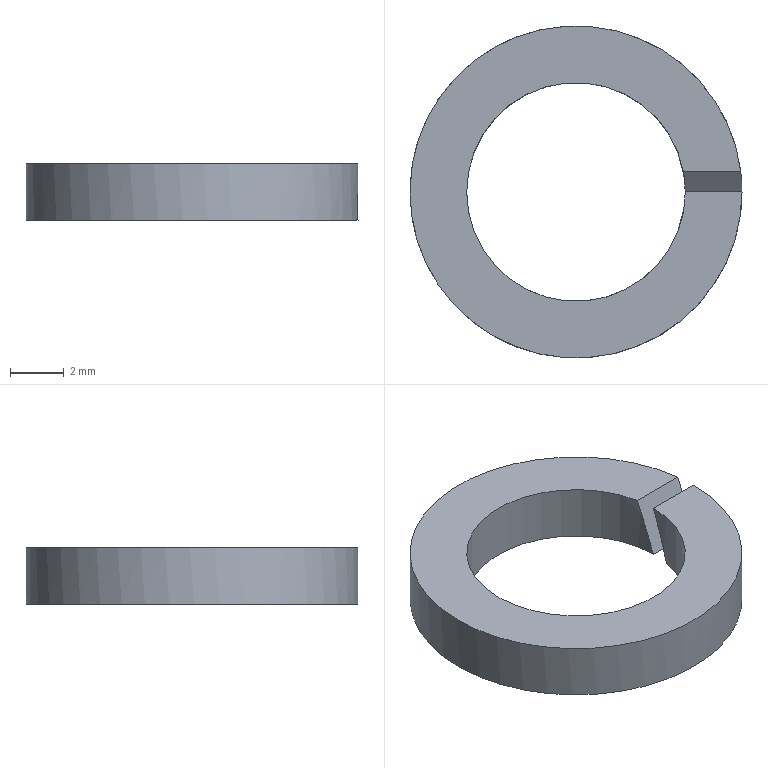Part | NX | features DATUM_CSYS 3, EXTRUDE 2, SKETCH 2 | 1 solid | 6 faces | box 12.3 x 12.3 x 2.1 mm | volume 137.929 mm3 | plane 4 | cylinder 2 | commonest cylinder face diameters 8.1 x1 12.3 x1
STEP:
#1=CARTESIAN_POINT('',(6.15,0.0009353,-1.05));
#2=VERTEX_POINT('',#1);
#3=CARTESIAN_POINT('',(6.102,0.7653,1.05));
#4=VERTEX_POINT('',#3);
#5=CARTESIAN_POINT('',(0.,0.,-1.053));
#6=DIRECTION('',(0.,-0.9397,0.342));
#7=DIRECTION('',(0.,-0.342,-0.9397));
#8=AXIS2_PLACEMENT_3D('',#5,#6,#7);
#9=ELLIPSE('',#8,17.981,6.15);
#10=EDGE_CURVE('',#2,#4,#9,.T.);
#11=ORIENTED_EDGE('',*,*,#10,.F.);
#12=CARTESIAN_POINT('',(6.102,-0.7653,-1.05));
#13=VERTEX_POINT('',#12);
#14=CARTESIAN_POINT('',(0.,0.,-1.05));
#15=DIRECTION('',(0.,0.,1.));
#16=DIRECTION('',(1.,0.,0.));
#17=AXIS2_PLACEMENT_3D('',#14,#15,#16);
#18=CIRCLE('',#17,6.15);
#19=EDGE_CURVE('',#2,#13,#18,.T.);
#20=ORIENTED_EDGE('',*,*,#19,.T.);
#21=CARTESIAN_POINT('',(6.15,-0.0009353,1.05));
#22=VERTEX_POINT('',#21);
#23=CARTESIAN_POINT('',(0.,0.,1.053));
#24=DIRECTION('',(0.,0.9397,-0.342));
#25=DIRECTION('',(0.,-0.342,-0.9397));
#26=AXIS2_PLACEMENT_3D('',#23,#24,#25);
#27=ELLIPSE('',#26,17.981,6.15);
#28=EDGE_CURVE('',#22,#13,#27,.T.);
#29=ORIENTED_EDGE('',*,*,#28,.F.);
#30=CARTESIAN_POINT('',(0.,0.,1.05));
#31=DIRECTION('',(0.,0.,1.));
#32=DIRECTION('',(1.,0.,0.));
#33=AXIS2_PLACEMENT_3D('',#30,#31,#32);
#34=CIRCLE('',#33,6.15);
#35=EDGE_CURVE('',#4,#22,#34,.T.);
#36=ORIENTED_EDGE('',*,*,#35,.F.);
#37=EDGE_LOOP('',(#11,#20,#29,#36));
#38=FACE_BOUND('',#37,.T.);
#39=CARTESIAN_POINT('',(0.,0.,1.05));
#40=DIRECTION('',(0.,0.,-1.));
#41=DIRECTION('',(-1.,0.,0.));
#42=AXIS2_PLACEMENT_3D('',#39,#40,#41);
#43=CYLINDRICAL_SURFACE('',#42,6.15);
#44=ADVANCED_FACE('',(#38),#43,.T.);
#45=CARTESIAN_POINT('',(4.05,0.0009353,-1.05));
#46=VERTEX_POINT('',#45);
#47=CARTESIAN_POINT('',(3.977,-0.7653,-1.05));
#48=VERTEX_POINT('',#47);
#49=CARTESIAN_POINT('',(0.,0.,-1.05));
#50=DIRECTION('',(0.,0.,1.));
#51=DIRECTION('',(1.,0.,0.));
#52=AXIS2_PLACEMENT_3D('',#49,#50,#51);
#53=CIRCLE('',#52,4.05);
#54=EDGE_CURVE('',#46,#48,#53,.T.);
#55=ORIENTED_EDGE('',*,*,#54,.F.);
#56=CARTESIAN_POINT('',(3.977,0.7653,1.05));
#57=VERTEX_POINT('',#56);
#58=CARTESIAN_POINT('',(0.,0.,-1.053));
#59=DIRECTION('',(0.,-0.9397,0.342));
#60=DIRECTION('',(0.,-0.342,-0.9397));
#61=AXIS2_PLACEMENT_3D('',#58,#59,#60);
#62=ELLIPSE('',#61,11.841,4.05);
#63=EDGE_CURVE('',#46,#57,#62,.T.);
#64=ORIENTED_EDGE('',*,*,#63,.T.);
#65=CARTESIAN_POINT('',(4.05,-0.0009353,1.05));
#66=VERTEX_POINT('',#65);
#67=CARTESIAN_POINT('',(0.,0.,1.05));
#68=DIRECTION('',(0.,0.,1.));
#69=DIRECTION('',(1.,0.,0.));
#70=AXIS2_PLACEMENT_3D('',#67,#68,#69);
#71=CIRCLE('',#70,4.05);
#72=EDGE_CURVE('',#57,#66,#71,.T.);
#73=ORIENTED_EDGE('',*,*,#72,.T.);
#74=CARTESIAN_POINT('',(0.,0.,1.053));
#75=DIRECTION('',(0.,0.9397,-0.342));
#76=DIRECTION('',(0.,-0.342,-0.9397));
#77=AXIS2_PLACEMENT_3D('',#74,#75,#76);
#78=ELLIPSE('',#77,11.841,4.05);
#79=EDGE_CURVE('',#66,#48,#78,.T.);
#80=ORIENTED_EDGE('',*,*,#79,.T.);
#81=EDGE_LOOP('',(#55,#64,#73,#80));
#82=FACE_BOUND('',#81,.T.);
#83=CARTESIAN_POINT('',(0.,0.,1.05));
#84=DIRECTION('',(0.,0.,-1.));
#85=DIRECTION('',(-1.,0.,0.));
#86=AXIS2_PLACEMENT_3D('',#83,#84,#85);
#87=CYLINDRICAL_SURFACE('',#86,4.05);
#88=ADVANCED_FACE('',(#82),#87,.F.);
#89=ORIENTED_EDGE('',*,*,#72,.F.);
#90=CARTESIAN_POINT('',(0.,0.7653,1.05));
#91=DIRECTION('',(1.,0.,0.));
#92=VECTOR('',#91,1000.);
#93=LINE('',#90,#92);
#94=EDGE_CURVE('',#57,#4,#93,.T.);
#95=ORIENTED_EDGE('',*,*,#94,.T.);
#96=ORIENTED_EDGE('',*,*,#35,.T.);
#97=CARTESIAN_POINT('',(0.,-0.0009353,1.05));
#98=DIRECTION('',(-1.,0.,0.));
#99=VECTOR('',#98,1000.);
#100=LINE('',#97,#99);
#101=EDGE_CURVE('',#22,#66,#100,.T.);
#102=ORIENTED_EDGE('',*,*,#101,.T.);
#103=EDGE_LOOP('',(#89,#95,#96,#102));
#104=FACE_BOUND('',#103,.T.);
#105=CARTESIAN_POINT('',(0.,0.,1.05));
#106=DIRECTION('',(0.,0.,1.));
#107=DIRECTION('',(1.,0.,0.));
#108=AXIS2_PLACEMENT_3D('',#105,#106,#107);
#109=PLANE('',#108);
#110=ADVANCED_FACE('',(#104),#109,.T.);
#111=CARTESIAN_POINT('',(0.,0.0009353,-1.05));
#112=DIRECTION('',(1.,0.,0.));
#113=VECTOR('',#112,1000.);
#114=LINE('',#111,#113);
#115=EDGE_CURVE('',#46,#2,#114,.T.);
#116=ORIENTED_EDGE('',*,*,#115,.F.);
#117=ORIENTED_EDGE('',*,*,#54,.T.);
#118=CARTESIAN_POINT('',(0.,-0.7653,-1.05));
#119=DIRECTION('',(-1.,0.,0.));
#120=VECTOR('',#119,1000.);
#121=LINE('',#118,#120);
#122=EDGE_CURVE('',#13,#48,#121,.T.);
#123=ORIENTED_EDGE('',*,*,#122,.F.);
#124=ORIENTED_EDGE('',*,*,#19,.F.);
#125=EDGE_LOOP('',(#116,#117,#123,#124));
#126=FACE_BOUND('',#125,.T.);
#127=CARTESIAN_POINT('',(0.,0.,-1.05));
#128=DIRECTION('',(0.,0.,1.));
#129=DIRECTION('',(1.,0.,0.));
#130=AXIS2_PLACEMENT_3D('',#127,#128,#129);
#131=PLANE('',#130);
#132=ADVANCED_FACE('',(#126),#131,.F.);
#133=ORIENTED_EDGE('',*,*,#28,.T.);
#134=ORIENTED_EDGE('',*,*,#122,.T.);
#135=ORIENTED_EDGE('',*,*,#79,.F.);
#136=ORIENTED_EDGE('',*,*,#101,.F.);
#137=EDGE_LOOP('',(#133,#134,#135,#136));
#138=FACE_BOUND('',#137,.T.);
#139=CARTESIAN_POINT('',(8.5,0.5266,2.499));
#140=DIRECTION('',(0.,0.9397,-0.342));
#141=DIRECTION('',(0.,0.342,0.9397));
#142=AXIS2_PLACEMENT_3D('',#139,#140,#141);
#143=PLANE('',#142);
#144=ADVANCED_FACE('',(#138),#143,.T.);
#145=ORIENTED_EDGE('',*,*,#63,.F.);
#146=ORIENTED_EDGE('',*,*,#115,.T.);
#147=ORIENTED_EDGE('',*,*,#10,.T.);
#148=ORIENTED_EDGE('',*,*,#94,.F.);
#149=EDGE_LOOP('',(#145,#146,#147,#148));
#150=FACE_BOUND('',#149,.T.);
#151=CARTESIAN_POINT('',(8.5,-0.5266,-2.499));
#152=DIRECTION('',(0.,-0.9397,0.342));
#153=DIRECTION('',(0.,-0.342,-0.9397));
#154=AXIS2_PLACEMENT_3D('',#151,#152,#153);
#155=PLANE('',#154);
#156=ADVANCED_FACE('',(#150),#155,.T.);
#157=CLOSED_SHELL('',(#44,#88,#110,#132,#144,#156));
#158=MANIFOLD_SOLID_BREP('',#157);
#159=(LENGTH_UNIT()NAMED_UNIT(*)SI_UNIT(.MILLI.,.METRE.));
#160=UNCERTAINTY_MEASURE_WITH_UNIT(LENGTH_MEASURE(0.00001),#159,'','');
#161=(NAMED_UNIT(*)PLANE_ANGLE_UNIT()SI_UNIT($,.RADIAN.));
#162=(NAMED_UNIT(*)SI_UNIT($,.STERADIAN.)SOLID_ANGLE_UNIT());
#163=(GEOMETRIC_REPRESENTATION_CONTEXT(3)GLOBAL_UNCERTAINTY_ASSIGNED_CONTEXT((#160))GLOBAL_UNIT_ASSIGNED_CONTEXT((#159,#161,#162))REPRESENTATION_CONTEXT('',''));
#164=ADVANCED_BREP_SHAPE_REPRESENTATION('',(#158),#163);